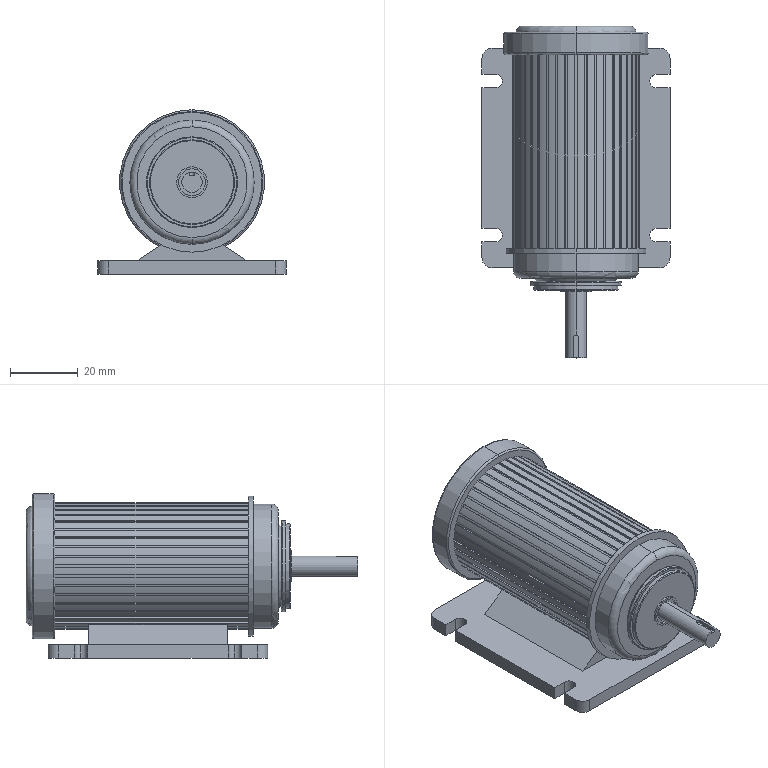Part | SolidWorks | features Cut 4, ICE 3, Extrusion 1, Fillet 1, Revolution 1 | 1 solid | 259 faces | box 55.501 x 97.908 x 48.521 mm | volume 103987 mm3 | plane 172 | cylinder 71 | torus 14 | cone 2 | commonest cylinder face diameters 37.3 x44 4 x6 6 x6 7.902 x2 9.067 x2 24.978 x2